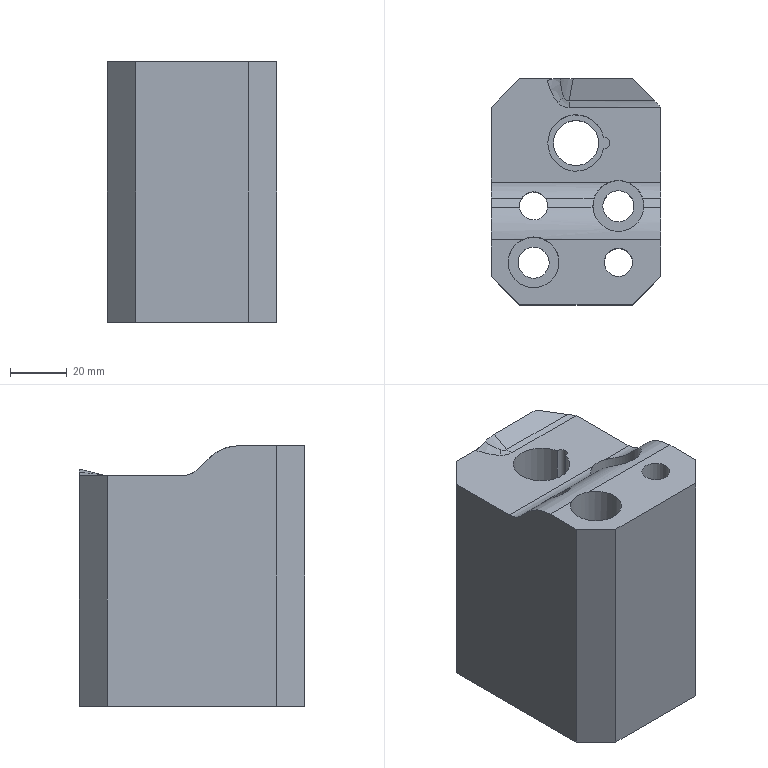Part | NX | features solid 2 | 1 solid | 37 faces | box 60 x 80 x 92.308 mm | volume 319167 mm3 | plane 19 | cylinder 15 | spline 3 | commonest cylinder face diameters 16 x3 20 x3 10 x2 11 x2 18 x2 4 x1
STEP:
#1=CARTESIAN_POINT('',(150.,-440.,5.));
#2=VERTEX_POINT('',#1);
#3=CARTESIAN_POINT('',(150.,-440.,97.308));
#4=VERTEX_POINT('',#3);
#5=CARTESIAN_POINT('',(150.,-440.,10.));
#6=DIRECTION('',(0.,0.,1.));
#7=VECTOR('',#6,1000.);
#8=LINE('',#5,#7);
#9=EDGE_CURVE('',#2,#4,#8,.T.);
#10=ORIENTED_EDGE('',*,*,#9,.T.);
#11=CARTESIAN_POINT('',(110.,-440.,97.308));
#12=VERTEX_POINT('',#11);
#13=CARTESIAN_POINT('',(130.,-440.,97.308));
#14=DIRECTION('',(-1.,0.,0.));
#15=VECTOR('',#14,1000.);
#16=LINE('',#13,#15);
#17=EDGE_CURVE('',#4,#12,#16,.T.);
#18=ORIENTED_EDGE('',*,*,#17,.T.);
#19=CARTESIAN_POINT('',(110.,-440.,5.));
#20=VERTEX_POINT('',#19);
#21=CARTESIAN_POINT('',(110.,-440.,10.));
#22=DIRECTION('',(0.,0.,-1.));
#23=VECTOR('',#22,1000.);
#24=LINE('',#21,#23);
#25=EDGE_CURVE('',#12,#20,#24,.T.);
#26=ORIENTED_EDGE('',*,*,#25,.T.);
#27=CARTESIAN_POINT('',(130.,-440.,5.));
#28=DIRECTION('',(-1.,0.,0.));
#29=VECTOR('',#28,1000.);
#30=LINE('',#27,#29);
#31=EDGE_CURVE('',#2,#20,#30,.T.);
#32=ORIENTED_EDGE('',*,*,#31,.F.);
#33=EDGE_LOOP('',(#10,#18,#26,#32));
#34=FACE_BOUND('',#33,.T.);
#35=CARTESIAN_POINT('',(130.,-440.,10.));
#36=DIRECTION('',(0.,-1.,0.));
#37=DIRECTION('',(0.,0.,-1.));
#38=AXIS2_PLACEMENT_3D('',#35,#36,#37);
#39=PLANE('',#38);
#40=ADVANCED_FACE('',(#34),#39,.T.);
#41=CARTESIAN_POINT('',(110.,-360.,5.));
#42=VERTEX_POINT('',#41);
#43=CARTESIAN_POINT('',(110.,-360.,86.708));
#44=VERTEX_POINT('',#43);
#45=CARTESIAN_POINT('',(110.,-360.,10.));
#46=DIRECTION('',(0.,0.,1.));
#47=VECTOR('',#46,1000.);
#48=LINE('',#45,#47);
#49=EDGE_CURVE('',#42,#44,#48,.T.);
#50=ORIENTED_EDGE('',*,*,#49,.T.);
#51=CARTESIAN_POINT('',(119.594,-360.,86.708));
#52=VERTEX_POINT('',#51);
#53=CARTESIAN_POINT('',(130.,-360.,86.708));
#54=DIRECTION('',(1.,0.,0.));
#55=VECTOR('',#54,1000.);
#56=LINE('',#53,#55);
#57=EDGE_CURVE('',#44,#52,#56,.T.);
#58=ORIENTED_EDGE('',*,*,#57,.T.);
#59=CARTESIAN_POINT('',(121.87,-360.,86.952));
#60=VERTEX_POINT('',#59);
#61=CARTESIAN_POINT('',(119.594,-360.,86.708));
#62=CARTESIAN_POINT('',(120.362,-360.,86.708));
#63=CARTESIAN_POINT('',(121.12,-360.,86.789));
#64=CARTESIAN_POINT('',(121.87,-360.,86.952));
#65=B_SPLINE_CURVE_WITH_KNOTS('',3,(#61,#62,#63,#64),.UNSPECIFIED.,.F.,.F.,(4,4),(0.,0.002289),.UNSPECIFIED.);
#66=EDGE_CURVE('',#52,#60,#65,.T.);
#67=ORIENTED_EDGE('',*,*,#66,.T.);
#68=CARTESIAN_POINT('',(124.411,-360.,87.846));
#69=VERTEX_POINT('',#68);
#70=CARTESIAN_POINT('',(121.87,-360.,86.952));
#71=CARTESIAN_POINT('',(122.751,-360.,87.142));
#72=CARTESIAN_POINT('',(123.605,-360.,87.443));
#73=CARTESIAN_POINT('',(124.411,-360.,87.846));
#74=B_SPLINE_CURVE_WITH_KNOTS('',3,(#70,#71,#72,#73),.UNSPECIFIED.,.F.,.F.,(4,4),(0.,0.002699),.UNSPECIFIED.);
#75=EDGE_CURVE('',#60,#69,#74,.T.);
#76=ORIENTED_EDGE('',*,*,#75,.T.);
#77=CARTESIAN_POINT('',(129.046,-360.,88.952));
#78=VERTEX_POINT('',#77);
#79=CARTESIAN_POINT('',(128.58,-360.,78.645));
#80=DIRECTION('',(0.,1.,0.));
#81=DIRECTION('',(0.6116,0.,0.7911));
#82=AXIS2_PLACEMENT_3D('',#79,#80,#81);
#83=ELLIPSE('',#82,10.485,10.);
#84=EDGE_CURVE('',#69,#78,#83,.T.);
#85=ORIENTED_EDGE('',*,*,#84,.T.);
#86=CARTESIAN_POINT('',(150.,-360.,88.952));
#87=VERTEX_POINT('',#86);
#88=CARTESIAN_POINT('',(130.,-360.,88.952));
#89=DIRECTION('',(-1.,0.,0.));
#90=VECTOR('',#89,1000.);
#91=LINE('',#88,#90);
#92=EDGE_CURVE('',#87,#78,#91,.T.);
#93=ORIENTED_EDGE('',*,*,#92,.F.);
#94=CARTESIAN_POINT('',(150.,-360.,5.));
#95=VERTEX_POINT('',#94);
#96=CARTESIAN_POINT('',(150.,-360.,10.));
#97=DIRECTION('',(0.,0.,-1.));
#98=VECTOR('',#97,1000.);
#99=LINE('',#96,#98);
#100=EDGE_CURVE('',#87,#95,#99,.T.);
#101=ORIENTED_EDGE('',*,*,#100,.T.);
#102=CARTESIAN_POINT('',(130.,-360.,5.));
#103=DIRECTION('',(1.,0.,0.));
#104=VECTOR('',#103,1000.);
#105=LINE('',#102,#104);
#106=EDGE_CURVE('',#42,#95,#105,.T.);
#107=ORIENTED_EDGE('',*,*,#106,.F.);
#108=EDGE_LOOP('',(#50,#58,#67,#76,#85,#93,#101,#107));
#109=FACE_BOUND('',#108,.T.);
#110=CARTESIAN_POINT('',(130.,-360.,10.));
#111=DIRECTION('',(0.,1.,0.));
#112=DIRECTION('',(0.,0.,1.));
#113=AXIS2_PLACEMENT_3D('',#110,#111,#112);
#114=PLANE('',#113);
#115=ADVANCED_FACE('',(#109),#114,.T.);
#116=CARTESIAN_POINT('',(100.,-430.,5.));
#117=VERTEX_POINT('',#116);
#118=CARTESIAN_POINT('',(100.,-430.,97.308));
#119=VERTEX_POINT('',#118);
#120=CARTESIAN_POINT('',(100.,-430.,10.));
#121=DIRECTION('',(0.,0.,1.));
#122=VECTOR('',#121,1000.);
#123=LINE('',#120,#122);
#124=EDGE_CURVE('',#117,#119,#123,.T.);
#125=ORIENTED_EDGE('',*,*,#124,.T.);
#126=CARTESIAN_POINT('',(100.,-417.041,97.308));
#127=VERTEX_POINT('',#126);
#128=CARTESIAN_POINT('',(100.,-360.,97.308));
#129=DIRECTION('',(0.,1.,0.));
#130=VECTOR('',#129,1000.);
#131=LINE('',#128,#130);
#132=EDGE_CURVE('',#119,#127,#131,.T.);
#133=ORIENTED_EDGE('',*,*,#132,.T.);
#134=CARTESIAN_POINT('',(100.,-405.652,92.546));
#135=VERTEX_POINT('',#134);
#136=CARTESIAN_POINT('',(100.,-417.041,81.308));
#137=DIRECTION('',(-1.,0.,0.));
#138=DIRECTION('',(0.,0.,1.));
#139=AXIS2_PLACEMENT_3D('',#136,#137,#138);
#140=CIRCLE('',#139,16.);
#141=EDGE_CURVE('',#127,#135,#140,.T.);
#142=ORIENTED_EDGE('',*,*,#141,.T.);
#143=CARTESIAN_POINT('',(100.,-402.24,89.089));
#144=VERTEX_POINT('',#143);
#145=CARTESIAN_POINT('',(100.,-341.861,27.899));
#146=DIRECTION('',(0.,-0.7024,0.7118));
#147=VECTOR('',#146,1000.);
#148=LINE('',#145,#147);
#149=EDGE_CURVE('',#144,#135,#148,.T.);
#150=ORIENTED_EDGE('',*,*,#149,.F.);
#151=CARTESIAN_POINT('',(100.,-396.546,86.708));
#152=VERTEX_POINT('',#151);
#153=CARTESIAN_POINT('',(100.,-396.546,94.708));
#154=DIRECTION('',(-1.,0.,0.));
#155=DIRECTION('',(0.,0.,1.));
#156=AXIS2_PLACEMENT_3D('',#153,#154,#155);
#157=CIRCLE('',#156,8.);
#158=EDGE_CURVE('',#152,#144,#157,.T.);
#159=ORIENTED_EDGE('',*,*,#158,.F.);
#160=CARTESIAN_POINT('',(100.,-370.,86.708));
#161=VERTEX_POINT('',#160);
#162=CARTESIAN_POINT('',(100.,-360.,86.708));
#163=DIRECTION('',(0.,1.,0.));
#164=VECTOR('',#163,1000.);
#165=LINE('',#162,#164);
#166=EDGE_CURVE('',#152,#161,#165,.T.);
#167=ORIENTED_EDGE('',*,*,#166,.T.);
#168=CARTESIAN_POINT('',(100.,-370.,5.));
#169=VERTEX_POINT('',#168);
#170=CARTESIAN_POINT('',(100.,-370.,10.));
#171=DIRECTION('',(0.,0.,-1.));
#172=VECTOR('',#171,1000.);
#173=LINE('',#170,#172);
#174=EDGE_CURVE('',#161,#169,#173,.T.);
#175=ORIENTED_EDGE('',*,*,#174,.T.);
#176=CARTESIAN_POINT('',(100.,-360.,5.));
#177=DIRECTION('',(0.,1.,0.));
#178=VECTOR('',#177,1000.);
#179=LINE('',#176,#178);
#180=EDGE_CURVE('',#117,#169,#179,.T.);
#181=ORIENTED_EDGE('',*,*,#180,.F.);
#182=EDGE_LOOP('',(#125,#133,#142,#150,#159,#167,#175,#181));
#183=FACE_BOUND('',#182,.T.);
#184=CARTESIAN_POINT('',(100.,-360.,10.));
#185=DIRECTION('',(-1.,0.,0.));
#186=DIRECTION('',(0.,0.,-1.));
#187=AXIS2_PLACEMENT_3D('',#184,#185,#186);
#188=PLANE('',#187);
#189=ADVANCED_FACE('',(#183),#188,.T.);
#190=ORIENTED_EDGE('',*,*,#174,.F.);
#191=CARTESIAN_POINT('',(110.,-360.,86.708));
#192=DIRECTION('',(-0.7071,-0.7071,0.));
#193=VECTOR('',#192,1000.);
#194=LINE('',#191,#193);
#195=EDGE_CURVE('',#161,#44,#194,.F.);
#196=ORIENTED_EDGE('',*,*,#195,.T.);
#197=ORIENTED_EDGE('',*,*,#49,.F.);
#198=CARTESIAN_POINT('',(120.,-350.,5.));
#199=DIRECTION('',(-0.7071,-0.7071,0.));
#200=VECTOR('',#199,1000.);
#201=LINE('',#198,#200);
#202=EDGE_CURVE('',#169,#42,#201,.F.);
#203=ORIENTED_EDGE('',*,*,#202,.F.);
#204=EDGE_LOOP('',(#190,#196,#197,#203));
#205=FACE_BOUND('',#204,.T.);
#206=CARTESIAN_POINT('',(110.,-360.,10.));
#207=DIRECTION('',(0.7071,-0.7071,0.));
#208=DIRECTION('',(0.7071,0.7071,0.));
#209=AXIS2_PLACEMENT_3D('',#206,#207,#208);
#210=PLANE('',#209);
#211=ADVANCED_FACE('',(#205),#210,.F.);
#212=CARTESIAN_POINT('',(160.,-430.,97.308));
#213=VERTEX_POINT('',#212);
#214=CARTESIAN_POINT('',(160.,-430.,5.));
#215=VERTEX_POINT('',#214);
#216=CARTESIAN_POINT('',(160.,-430.,10.));
#217=DIRECTION('',(0.,0.,-1.));
#218=VECTOR('',#217,1000.);
#219=LINE('',#216,#218);
#220=EDGE_CURVE('',#213,#215,#219,.T.);
#221=ORIENTED_EDGE('',*,*,#220,.F.);
#222=CARTESIAN_POINT('',(150.,-440.,97.308));
#223=DIRECTION('',(0.7071,0.7071,0.));
#224=VECTOR('',#223,1000.);
#225=LINE('',#222,#224);
#226=EDGE_CURVE('',#213,#4,#225,.F.);
#227=ORIENTED_EDGE('',*,*,#226,.T.);
#228=ORIENTED_EDGE('',*,*,#9,.F.);
#229=CARTESIAN_POINT('',(180.,-410.,5.));
#230=DIRECTION('',(0.7071,0.7071,0.));
#231=VECTOR('',#230,1000.);
#232=LINE('',#229,#231);
#233=EDGE_CURVE('',#215,#2,#232,.F.);
#234=ORIENTED_EDGE('',*,*,#233,.F.);
#235=EDGE_LOOP('',(#221,#227,#228,#234));
#236=FACE_BOUND('',#235,.T.);
#237=CARTESIAN_POINT('',(150.,-440.,10.));
#238=DIRECTION('',(-0.7071,0.7071,0.));
#239=DIRECTION('',(-0.7071,-0.7071,0.));
#240=AXIS2_PLACEMENT_3D('',#237,#238,#239);
#241=PLANE('',#240);
#242=ADVANCED_FACE('',(#236),#241,.F.);
#243=ORIENTED_EDGE('',*,*,#25,.F.);
#244=CARTESIAN_POINT('',(100.,-430.,97.308));
#245=DIRECTION('',(0.7071,-0.7071,0.));
#246=VECTOR('',#245,1000.);
#247=LINE('',#244,#246);
#248=EDGE_CURVE('',#12,#119,#247,.F.);
#249=ORIENTED_EDGE('',*,*,#248,.T.);
#250=ORIENTED_EDGE('',*,*,#124,.F.);
#251=CARTESIAN_POINT('',(80.,-410.,5.));
#252=DIRECTION('',(0.7071,-0.7071,0.));
#253=VECTOR('',#252,1000.);
#254=LINE('',#251,#253);
#255=EDGE_CURVE('',#20,#117,#254,.F.);
#256=ORIENTED_EDGE('',*,*,#255,.F.);
#257=EDGE_LOOP('',(#243,#249,#250,#256));
#258=FACE_BOUND('',#257,.T.);
#259=CARTESIAN_POINT('',(100.,-430.,10.));
#260=DIRECTION('',(0.7071,0.7071,0.));
#261=DIRECTION('',(-0.7071,0.7071,0.));
#262=AXIS2_PLACEMENT_3D('',#259,#260,#261);
#263=PLANE('',#262);
#264=ADVANCED_FACE('',(#258),#263,.F.);
#265=CARTESIAN_POINT('',(106.,-425.,35.));
#266=VERTEX_POINT('',#265);
#267=CARTESIAN_POINT('',(115.,-425.,35.));
#268=DIRECTION('',(0.,0.,-1.));
#269=DIRECTION('',(-1.,0.,0.));
#270=AXIS2_PLACEMENT_3D('',#267,#268,#269);
#271=CIRCLE('',#270,9.);
#272=EDGE_CURVE('',#266,#266,#271,.T.);
#273=ORIENTED_EDGE('',*,*,#272,.T.);
#274=EDGE_LOOP('',(#273));
#275=FACE_BOUND('',#274,.T.);
#276=CARTESIAN_POINT('',(119.201,-417.041,97.308));
#277=VERTEX_POINT('',#276);
#278=CARTESIAN_POINT('',(110.799,-417.041,97.308));
#279=VERTEX_POINT('',#278);
#280=CARTESIAN_POINT('',(115.,-425.,97.308));
#281=DIRECTION('',(0.,0.,1.));
#282=DIRECTION('',(1.,0.,0.));
#283=AXIS2_PLACEMENT_3D('',#280,#281,#282);
#284=CIRCLE('',#283,9.);
#285=EDGE_CURVE('',#277,#279,#284,.F.);
#286=ORIENTED_EDGE('',*,*,#285,.F.);
#287=CARTESIAN_POINT('',(110.799,-417.041,97.308));
#288=CARTESIAN_POINT('',(112.099,-416.354,97.308));
#289=CARTESIAN_POINT('',(114.996,-415.646,97.24));
#290=CARTESIAN_POINT('',(117.901,-416.354,97.308));
#291=CARTESIAN_POINT('',(119.201,-417.041,97.308));
#292=B_SPLINE_CURVE_WITH_KNOTS('',3,(#287,#288,#289,#290,#291),.UNSPECIFIED.,.F.,.F.,(4,1,4),(0.,0.004347,0.008695),.UNSPECIFIED.);
#293=EDGE_CURVE('',#279,#277,#292,.T.);
#294=ORIENTED_EDGE('',*,*,#293,.F.);
#295=EDGE_LOOP('',(#286,#294));
#296=FACE_BOUND('',#295,.T.);
#297=CARTESIAN_POINT('',(115.,-425.,110.));
#298=DIRECTION('',(0.,0.,-1.));
#299=DIRECTION('',(-1.,0.,0.));
#300=AXIS2_PLACEMENT_3D('',#297,#298,#299);
#301=CYLINDRICAL_SURFACE('',#300,9.);
#302=ADVANCED_FACE('',(#275,#296),#301,.F.);
#303=CARTESIAN_POINT('',(140.,-425.,5.));
#304=VERTEX_POINT('',#303);
#305=CARTESIAN_POINT('',(145.,-425.,5.));
#306=DIRECTION('',(0.,0.,-1.));
#307=DIRECTION('',(-1.,0.,0.));
#308=AXIS2_PLACEMENT_3D('',#305,#306,#307);
#309=CIRCLE('',#308,5.);
#310=EDGE_CURVE('',#304,#304,#309,.T.);
#311=ORIENTED_EDGE('',*,*,#310,.T.);
#312=EDGE_LOOP('',(#311));
#313=FACE_BOUND('',#312,.T.);
#314=CARTESIAN_POINT('',(150.,-425.,97.308));
#315=VERTEX_POINT('',#314);
#316=CARTESIAN_POINT('',(145.,-425.,97.308));
#317=DIRECTION('',(0.,0.,1.));
#318=DIRECTION('',(1.,0.,0.));
#319=AXIS2_PLACEMENT_3D('',#316,#317,#318);
#320=CIRCLE('',#319,5.);
#321=EDGE_CURVE('',#315,#315,#320,.F.);
#322=ORIENTED_EDGE('',*,*,#321,.F.);
#323=EDGE_LOOP('',(#322));
#324=FACE_BOUND('',#323,.T.);
#325=CARTESIAN_POINT('',(145.,-425.,110.));
#326=DIRECTION('',(0.,0.,-1.));
#327=DIRECTION('',(-1.,0.,0.));
#328=AXIS2_PLACEMENT_3D('',#325,#326,#327);
#329=CYLINDRICAL_SURFACE('',#328,5.);
#330=ADVANCED_FACE('',(#313,#324),#329,.F.);
#331=CARTESIAN_POINT('',(160.,-370.228,86.708));
#332=VERTEX_POINT('',#331);
#333=CARTESIAN_POINT('',(160.,-370.,86.71));
#334=VERTEX_POINT('',#333);
#335=CARTESIAN_POINT('',(160.,-370.228,96.708));
#336=DIRECTION('',(1.,0.,0.));
#337=DIRECTION('',(0.,0.,-1.));
#338=AXIS2_PLACEMENT_3D('',#335,#336,#337);
#339=CIRCLE('',#338,10.);
#340=EDGE_CURVE('',#332,#334,#339,.T.);
#341=ORIENTED_EDGE('',*,*,#340,.F.);
#342=CARTESIAN_POINT('',(160.,-396.546,86.708));
#343=VERTEX_POINT('',#342);
#344=CARTESIAN_POINT('',(160.,-360.,86.708));
#345=DIRECTION('',(0.,-1.,0.));
#346=VECTOR('',#345,1000.);
#347=LINE('',#344,#346);
#348=EDGE_CURVE('',#332,#343,#347,.T.);
#349=ORIENTED_EDGE('',*,*,#348,.T.);
#350=CARTESIAN_POINT('',(160.,-402.24,89.089));
#351=VERTEX_POINT('',#350);
#352=CARTESIAN_POINT('',(160.,-396.546,94.708));
#353=DIRECTION('',(1.,0.,0.));
#354=DIRECTION('',(0.,0.,-1.));
#355=AXIS2_PLACEMENT_3D('',#352,#353,#354);
#356=CIRCLE('',#355,8.);
#357=EDGE_CURVE('',#351,#343,#356,.T.);
#358=ORIENTED_EDGE('',*,*,#357,.F.);
#359=CARTESIAN_POINT('',(160.,-405.652,92.546));
#360=VERTEX_POINT('',#359);
#361=CARTESIAN_POINT('',(160.,-341.861,27.899));
#362=DIRECTION('',(0.,0.7024,-0.7118));
#363=VECTOR('',#362,1000.);
#364=LINE('',#361,#363);
#365=EDGE_CURVE('',#360,#351,#364,.T.);
#366=ORIENTED_EDGE('',*,*,#365,.F.);
#367=CARTESIAN_POINT('',(160.,-417.041,97.308));
#368=VERTEX_POINT('',#367);
#369=CARTESIAN_POINT('',(160.,-417.041,81.308));
#370=DIRECTION('',(1.,0.,0.));
#371=DIRECTION('',(0.,0.,-1.));
#372=AXIS2_PLACEMENT_3D('',#369,#370,#371);
#373=CIRCLE('',#372,16.);
#374=EDGE_CURVE('',#360,#368,#373,.T.);
#375=ORIENTED_EDGE('',*,*,#374,.T.);
#376=CARTESIAN_POINT('',(160.,-360.,97.308));
#377=DIRECTION('',(0.,-1.,0.));
#378=VECTOR('',#377,1000.);
#379=LINE('',#376,#378);
#380=EDGE_CURVE('',#368,#213,#379,.T.);
#381=ORIENTED_EDGE('',*,*,#380,.T.);
#382=ORIENTED_EDGE('',*,*,#220,.T.);
#383=CARTESIAN_POINT('',(160.,-370.,5.));
#384=VERTEX_POINT('',#383);
#385=CARTESIAN_POINT('',(160.,-360.,5.));
#386=DIRECTION('',(0.,-1.,0.));
#387=VECTOR('',#386,1000.);
#388=LINE('',#385,#387);
#389=EDGE_CURVE('',#384,#215,#388,.T.);
#390=ORIENTED_EDGE('',*,*,#389,.F.);
#391=CARTESIAN_POINT('',(160.,-370.,10.));
#392=DIRECTION('',(0.,0.,1.));
#393=VECTOR('',#392,1000.);
#394=LINE('',#391,#393);
#395=EDGE_CURVE('',#384,#334,#394,.T.);
#396=ORIENTED_EDGE('',*,*,#395,.T.);
#397=EDGE_LOOP('',(#341,#349,#358,#366,#375,#381,#382,#390,#396));
#398=FACE_BOUND('',#397,.T.);
#399=CARTESIAN_POINT('',(160.,-360.,10.));
#400=DIRECTION('',(1.,0.,0.));
#401=DIRECTION('',(0.,0.,1.));
#402=AXIS2_PLACEMENT_3D('',#399,#400,#401);
#403=PLANE('',#402);
#404=ADVANCED_FACE('',(#398),#403,.T.);
#405=CARTESIAN_POINT('',(118.511,-382.715,5.));
#406=VERTEX_POINT('',#405);
#407=CARTESIAN_POINT('',(130.011,-382.715,5.));
#408=DIRECTION('',(0.,0.,-1.));
#409=DIRECTION('',(-1.,0.,0.));
#410=AXIS2_PLACEMENT_3D('',#407,#408,#409);
#411=CIRCLE('',#410,11.5);
#412=EDGE_CURVE('',#406,#406,#411,.F.);
#413=ORIENTED_EDGE('',*,*,#412,.T.);
#414=EDGE_LOOP('',(#413));
#415=FACE_BOUND('',#414,.T.);
#416=ORIENTED_EDGE('',*,*,#310,.F.);
#417=EDGE_LOOP('',(#416));
#418=FACE_BOUND('',#417,.T.);
#419=CARTESIAN_POINT('',(110.,-405.,5.));
#420=VERTEX_POINT('',#419);
#421=CARTESIAN_POINT('',(115.,-405.,5.));
#422=DIRECTION('',(0.,0.,-1.));
#423=DIRECTION('',(-1.,0.,0.));
#424=AXIS2_PLACEMENT_3D('',#421,#422,#423);
#425=CIRCLE('',#424,5.);
#426=EDGE_CURVE('',#420,#420,#425,.T.);
#427=ORIENTED_EDGE('',*,*,#426,.F.);
#428=EDGE_LOOP('',(#427));
#429=FACE_BOUND('',#428,.T.);
#430=CARTESIAN_POINT('',(139.5,-405.,5.));
#431=VERTEX_POINT('',#430);
#432=CARTESIAN_POINT('',(145.,-405.,5.));
#433=DIRECTION('',(0.,0.,-1.));
#434=DIRECTION('',(-1.,0.,0.));
#435=AXIS2_PLACEMENT_3D('',#432,#433,#434);
#436=CIRCLE('',#435,5.5);
#437=EDGE_CURVE('',#431,#431,#436,.T.);
#438=ORIENTED_EDGE('',*,*,#437,.F.);
#439=EDGE_LOOP('',(#438));
#440=FACE_BOUND('',#439,.T.);
#441=CARTESIAN_POINT('',(109.5,-425.,5.));
#442=VERTEX_POINT('',#441);
#443=CARTESIAN_POINT('',(115.,-425.,5.));
#444=DIRECTION('',(0.,0.,-1.));
#445=DIRECTION('',(-1.,0.,0.));
#446=AXIS2_PLACEMENT_3D('',#443,#444,#445);
#447=CIRCLE('',#446,5.5);
#448=EDGE_CURVE('',#442,#442,#447,.T.);
#449=ORIENTED_EDGE('',*,*,#448,.F.);
#450=EDGE_LOOP('',(#449));
#451=FACE_BOUND('',#450,.T.);
#452=ORIENTED_EDGE('',*,*,#180,.T.);
#453=ORIENTED_EDGE('',*,*,#202,.T.);
#454=ORIENTED_EDGE('',*,*,#106,.T.);
#455=CARTESIAN_POINT('',(140.,-350.,5.));
#456=DIRECTION('',(-0.7071,0.7071,0.));
#457=VECTOR('',#456,1000.);
#458=LINE('',#455,#457);
#459=EDGE_CURVE('',#95,#384,#458,.F.);
#460=ORIENTED_EDGE('',*,*,#459,.T.);
#461=ORIENTED_EDGE('',*,*,#389,.T.);
#462=ORIENTED_EDGE('',*,*,#233,.T.);
#463=ORIENTED_EDGE('',*,*,#31,.T.);
#464=ORIENTED_EDGE('',*,*,#255,.T.);
#465=EDGE_LOOP('',(#452,#453,#454,#460,#461,#462,#463,#464));
#466=FACE_BOUND('',#465,.T.);
#467=CARTESIAN_POINT('',(130.,-360.,5.));
#468=DIRECTION('',(0.,0.,-1.));
#469=DIRECTION('',(1.,0.,0.));
#470=AXIS2_PLACEMENT_3D('',#467,#468,#469);
#471=PLANE('',#470);
#472=ADVANCED_FACE('',(#415,#418,#429,#440,#451,#466),#471,.T.);
#473=CARTESIAN_POINT('',(157.809,-367.809,87.005));
#474=VERTEX_POINT('',#473);
#475=CARTESIAN_POINT('',(160.228,-370.228,96.708));
#476=DIRECTION('',(-0.7071,-0.7071,0.));
#477=DIRECTION('',(-0.7071,0.7071,0.));
#478=AXIS2_PLACEMENT_3D('',#475,#476,#477);
#479=ELLIPSE('',#478,14.142,10.);
#480=EDGE_CURVE('',#334,#474,#479,.F.);
#481=ORIENTED_EDGE('',*,*,#480,.F.);
#482=ORIENTED_EDGE('',*,*,#395,.F.);
#483=ORIENTED_EDGE('',*,*,#459,.F.);
#484=ORIENTED_EDGE('',*,*,#100,.F.);
#485=CARTESIAN_POINT('',(169.244,-379.244,84.153));
#486=DIRECTION('',(0.6964,-0.6964,-0.1736));
#487=VECTOR('',#486,1000.);
#488=LINE('',#485,#487);
#489=EDGE_CURVE('',#474,#87,#488,.F.);
#490=ORIENTED_EDGE('',*,*,#489,.F.);
#491=EDGE_LOOP('',(#481,#482,#483,#484,#490));
#492=FACE_BOUND('',#491,.T.);
#493=CARTESIAN_POINT('',(160.,-370.,10.));
#494=DIRECTION('',(-0.7071,-0.7071,0.));
#495=DIRECTION('',(0.7071,-0.7071,0.));
#496=AXIS2_PLACEMENT_3D('',#493,#494,#495);
#497=PLANE('',#496);
#498=ADVANCED_FACE('',(#492),#497,.F.);
#499=ORIENTED_EDGE('',*,*,#448,.T.);
#500=EDGE_LOOP('',(#499));
#501=FACE_BOUND('',#500,.T.);
#502=CARTESIAN_POINT('',(109.5,-425.,35.));
#503=VERTEX_POINT('',#502);
#504=CARTESIAN_POINT('',(115.,-425.,35.));
#505=DIRECTION('',(0.,0.,-1.));
#506=DIRECTION('',(-1.,0.,0.));
#507=AXIS2_PLACEMENT_3D('',#504,#505,#506);
#508=CIRCLE('',#507,5.5);
#509=EDGE_CURVE('',#503,#503,#508,.T.);
#510=ORIENTED_EDGE('',*,*,#509,.F.);
#511=EDGE_LOOP('',(#510));
#512=FACE_BOUND('',#511,.T.);
#513=CARTESIAN_POINT('',(115.,-425.,5.));
#514=DIRECTION('',(0.,0.,-1.));
#515=DIRECTION('',(-1.,0.,0.));
#516=AXIS2_PLACEMENT_3D('',#513,#514,#515);
#517=CYLINDRICAL_SURFACE('',#516,5.5);
#518=ADVANCED_FACE('',(#501,#512),#517,.F.);
#519=ORIENTED_EDGE('',*,*,#509,.T.);
#520=EDGE_LOOP('',(#519));
#521=FACE_BOUND('',#520,.T.);
#522=ORIENTED_EDGE('',*,*,#272,.F.);
#523=EDGE_LOOP('',(#522));
#524=FACE_BOUND('',#523,.T.);
#525=CARTESIAN_POINT('',(115.,-425.,35.));
#526=DIRECTION('',(0.,0.,-1.));
#527=DIRECTION('',(-1.,0.,0.));
#528=AXIS2_PLACEMENT_3D('',#525,#526,#527);
#529=PLANE('',#528);
#530=ADVANCED_FACE('',(#521,#524),#529,.F.);
#531=ORIENTED_EDGE('',*,*,#437,.T.);
#532=EDGE_LOOP('',(#531));
#533=FACE_BOUND('',#532,.T.);
#534=CARTESIAN_POINT('',(139.5,-405.,35.));
#535=VERTEX_POINT('',#534);
#536=CARTESIAN_POINT('',(145.,-405.,35.));
#537=DIRECTION('',(0.,0.,-1.));
#538=DIRECTION('',(-1.,0.,0.));
#539=AXIS2_PLACEMENT_3D('',#536,#537,#538);
#540=CIRCLE('',#539,5.5);
#541=EDGE_CURVE('',#535,#535,#540,.T.);
#542=ORIENTED_EDGE('',*,*,#541,.F.);
#543=EDGE_LOOP('',(#542));
#544=FACE_BOUND('',#543,.T.);
#545=CARTESIAN_POINT('',(145.,-405.,5.));
#546=DIRECTION('',(0.,0.,-1.));
#547=DIRECTION('',(-1.,0.,0.));
#548=AXIS2_PLACEMENT_3D('',#545,#546,#547);
#549=CYLINDRICAL_SURFACE('',#548,5.5);
#550=ADVANCED_FACE('',(#533,#544),#549,.F.);
#551=ORIENTED_EDGE('',*,*,#541,.T.);
#552=EDGE_LOOP('',(#551));
#553=FACE_BOUND('',#552,.T.);
#554=CARTESIAN_POINT('',(136.,-405.,35.));
#555=VERTEX_POINT('',#554);
#556=CARTESIAN_POINT('',(145.,-405.,35.));
#557=DIRECTION('',(0.,0.,-1.));
#558=DIRECTION('',(-1.,0.,0.));
#559=AXIS2_PLACEMENT_3D('',#556,#557,#558);
#560=CIRCLE('',#559,9.);
#561=EDGE_CURVE('',#555,#555,#560,.T.);
#562=ORIENTED_EDGE('',*,*,#561,.F.);
#563=EDGE_LOOP('',(#562));
#564=FACE_BOUND('',#563,.T.);
#565=CARTESIAN_POINT('',(145.,-405.,35.));
#566=DIRECTION('',(0.,0.,-1.));
#567=DIRECTION('',(-1.,0.,0.));
#568=AXIS2_PLACEMENT_3D('',#565,#566,#567);
#569=PLANE('',#568);
#570=ADVANCED_FACE('',(#553,#564),#569,.F.);
#571=CARTESIAN_POINT('',(141.913,-396.546,86.708));
#572=VERTEX_POINT('',#571);
#573=CARTESIAN_POINT('',(148.087,-396.546,86.708));
#574=VERTEX_POINT('',#573);
#575=CARTESIAN_POINT('',(145.,-405.,86.708));
#576=DIRECTION('',(0.,0.,1.));
#577=DIRECTION('',(1.,0.,0.));
#578=AXIS2_PLACEMENT_3D('',#575,#576,#577);
#579=CIRCLE('',#578,9.);
#580=EDGE_CURVE('',#572,#574,#579,.F.);
#581=ORIENTED_EDGE('',*,*,#580,.F.);
#582=CARTESIAN_POINT('',(136.434,-402.24,89.089));
#583=VERTEX_POINT('',#582);
#584=CARTESIAN_POINT('',(141.913,-396.546,86.708));
#585=CARTESIAN_POINT('',(140.531,-397.051,86.708));
#586=CARTESIAN_POINT('',(138.034,-398.754,86.767));
#587=CARTESIAN_POINT('',(136.759,-401.229,88.064));
#588=CARTESIAN_POINT('',(136.434,-402.24,89.089));
#589=B_SPLINE_CURVE_WITH_KNOTS('',3,(#584,#585,#586,#587,#588),.UNSPECIFIED.,.F.,.F.,(4,1,4),(0.,0.004358,0.008716),.UNSPECIFIED.);
#590=EDGE_CURVE('',#572,#583,#589,.T.);
#591=ORIENTED_EDGE('',*,*,#590,.T.);
#592=CARTESIAN_POINT('',(136.024,-405.652,92.546));
#593=VERTEX_POINT('',#592);
#594=CARTESIAN_POINT('',(145.,-405.,91.885));
#595=DIRECTION('',(0.,-0.7118,-0.7024));
#596=DIRECTION('',(0.,0.7024,-0.7118));
#597=AXIS2_PLACEMENT_3D('',#594,#595,#596);
#598=ELLIPSE('',#597,12.814,9.);
#599=EDGE_CURVE('',#583,#593,#598,.F.);
#600=ORIENTED_EDGE('',*,*,#599,.T.);
#601=CARTESIAN_POINT('',(153.976,-405.652,92.546));
#602=VERTEX_POINT('',#601);
#603=CARTESIAN_POINT('',(153.976,-405.652,92.546));
#604=CARTESIAN_POINT('',(153.914,-406.513,93.419));
#605=CARTESIAN_POINT('',(153.527,-408.421,94.941));
#606=CARTESIAN_POINT('',(151.701,-411.359,96.352));
#607=CARTESIAN_POINT('',(148.672,-413.492,96.93));
#608=CARTESIAN_POINT('',(145.017,-414.251,97.058));
#609=CARTESIAN_POINT('',(141.353,-413.503,96.933));
#610=CARTESIAN_POINT('',(138.315,-411.377,96.358));
#611=CARTESIAN_POINT('',(136.476,-408.434,94.95));
#612=CARTESIAN_POINT('',(136.086,-406.514,93.42));
#613=CARTESIAN_POINT('',(136.024,-405.652,92.546));
#614=B_SPLINE_CURVE_WITH_KNOTS('',3,(#603,#604,#605,#606,#607,#608,#609,#610,#611,#612,#613),.UNSPECIFIED.,.F.,.F.,(4,1,1,1,1,1,1,1,4),(0.,0.003639,0.007278,0.01092,0.01456,0.01819,0.02183,0.02547,0.02911),.UNSPECIFIED.);
#615=EDGE_CURVE('',#602,#593,#614,.T.);
#616=ORIENTED_EDGE('',*,*,#615,.F.);
#617=CARTESIAN_POINT('',(153.566,-402.24,89.089));
#618=VERTEX_POINT('',#617);
#619=CARTESIAN_POINT('',(145.,-405.,91.885));
#620=DIRECTION('',(0.,-0.7118,-0.7024));
#621=DIRECTION('',(0.,0.7024,-0.7118));
#622=AXIS2_PLACEMENT_3D('',#619,#620,#621);
#623=ELLIPSE('',#622,12.814,9.);
#624=EDGE_CURVE('',#602,#618,#623,.F.);
#625=ORIENTED_EDGE('',*,*,#624,.T.);
#626=CARTESIAN_POINT('',(153.566,-402.24,89.089));
#627=CARTESIAN_POINT('',(153.242,-401.232,88.067));
#628=CARTESIAN_POINT('',(151.982,-398.77,86.771));
#629=CARTESIAN_POINT('',(149.467,-397.05,86.708));
#630=CARTESIAN_POINT('',(148.087,-396.546,86.708));
#631=B_SPLINE_CURVE_WITH_KNOTS('',3,(#626,#627,#628,#629,#630),.UNSPECIFIED.,.F.,.F.,(4,1,4),(0.,0.004352,0.008704),.UNSPECIFIED.);
#632=EDGE_CURVE('',#618,#574,#631,.T.);
#633=ORIENTED_EDGE('',*,*,#632,.T.);
#634=EDGE_LOOP('',(#581,#591,#600,#616,#625,#633));
#635=FACE_BOUND('',#634,.T.);
#636=ORIENTED_EDGE('',*,*,#561,.T.);
#637=EDGE_LOOP('',(#636));
#638=FACE_BOUND('',#637,.T.);
#639=CARTESIAN_POINT('',(145.,-405.,110.));
#640=DIRECTION('',(0.,0.,-1.));
#641=DIRECTION('',(-1.,0.,0.));
#642=AXIS2_PLACEMENT_3D('',#639,#640,#641);
#643=CYLINDRICAL_SURFACE('',#642,9.);
#644=ADVANCED_FACE('',(#635,#638),#643,.F.);
#645=CARTESIAN_POINT('',(119.169,-402.24,89.089));
#646=VERTEX_POINT('',#645);
#647=CARTESIAN_POINT('',(110.831,-402.24,89.089));
#648=VERTEX_POINT('',#647);
#649=CARTESIAN_POINT('',(119.169,-402.24,89.089));
#650=CARTESIAN_POINT('',(118.794,-401.674,88.514));
#651=CARTESIAN_POINT('',(117.655,-400.5,87.7));
#652=CARTESIAN_POINT('',(115.,-399.751,87.388));
#653=CARTESIAN_POINT('',(112.348,-400.498,87.699));
#654=CARTESIAN_POINT('',(111.206,-401.674,88.514));
#655=CARTESIAN_POINT('',(110.831,-402.24,89.089));
#656=B_SPLINE_CURVE_WITH_KNOTS('',3,(#649,#650,#651,#652,#653,#654,#655),.UNSPECIFIED.,.F.,.F.,(4,1,1,1,4),(0.,0.002634,0.005268,0.007902,0.01054),.UNSPECIFIED.);
#657=EDGE_CURVE('',#646,#648,#656,.T.);
#658=ORIENTED_EDGE('',*,*,#657,.T.);
#659=CARTESIAN_POINT('',(110.043,-405.652,92.546));
#660=VERTEX_POINT('',#659);
#661=CARTESIAN_POINT('',(115.,-405.,91.885));
#662=DIRECTION('',(0.,-0.7118,-0.7024));
#663=DIRECTION('',(0.,0.7024,-0.7118));
#664=AXIS2_PLACEMENT_3D('',#661,#662,#663);
#665=ELLIPSE('',#664,7.119,5.);
#666=EDGE_CURVE('',#648,#660,#665,.F.);
#667=ORIENTED_EDGE('',*,*,#666,.T.);
#668=CARTESIAN_POINT('',(119.957,-405.652,92.546));
#669=VERTEX_POINT('',#668);
#670=CARTESIAN_POINT('',(119.957,-405.652,92.546));
#671=CARTESIAN_POINT('',(119.833,-406.597,93.504));
#672=CARTESIAN_POINT('',(118.997,-408.762,95.124));
#673=CARTESIAN_POINT('',(115.011,-410.615,95.949));
#674=CARTESIAN_POINT('',(111.015,-408.779,95.134));
#675=CARTESIAN_POINT('',(110.167,-406.599,93.506));
#676=CARTESIAN_POINT('',(110.043,-405.652,92.546));
#677=B_SPLINE_CURVE_WITH_KNOTS('',3,(#670,#671,#672,#673,#674,#675,#676),.UNSPECIFIED.,.F.,.F.,(4,1,1,1,4),(0.,0.003993,0.007986,0.01198,0.01597),.UNSPECIFIED.);
#678=EDGE_CURVE('',#669,#660,#677,.T.);
#679=ORIENTED_EDGE('',*,*,#678,.F.);
#680=CARTESIAN_POINT('',(115.,-405.,91.885));
#681=DIRECTION('',(0.,-0.7118,-0.7024));
#682=DIRECTION('',(0.,0.7024,-0.7118));
#683=AXIS2_PLACEMENT_3D('',#680,#681,#682);
#684=ELLIPSE('',#683,7.119,5.);
#685=EDGE_CURVE('',#669,#646,#684,.F.);
#686=ORIENTED_EDGE('',*,*,#685,.T.);
#687=EDGE_LOOP('',(#658,#667,#679,#686));
#688=FACE_BOUND('',#687,.T.);
#689=ORIENTED_EDGE('',*,*,#426,.T.);
#690=EDGE_LOOP('',(#689));
#691=FACE_BOUND('',#690,.T.);
#692=CARTESIAN_POINT('',(115.,-405.,110.));
#693=DIRECTION('',(0.,0.,-1.));
#694=DIRECTION('',(-1.,0.,0.));
#695=AXIS2_PLACEMENT_3D('',#692,#693,#694);
#696=CYLINDRICAL_SURFACE('',#695,5.);
#697=ADVANCED_FACE('',(#688,#691),#696,.F.);
#698=CARTESIAN_POINT('',(139.811,-384.705,86.708));
#699=VERTEX_POINT('',#698);
#700=CARTESIAN_POINT('',(139.811,-380.725,86.708));
#701=VERTEX_POINT('',#700);
#702=CARTESIAN_POINT('',(140.011,-382.715,86.708));
#703=DIRECTION('',(0.,0.,1.));
#704=DIRECTION('',(1.,0.,0.));
#705=AXIS2_PLACEMENT_3D('',#702,#703,#704);
#706=CIRCLE('',#705,2.);
#707=EDGE_CURVE('',#699,#701,#706,.T.);
#708=ORIENTED_EDGE('',*,*,#707,.F.);
#709=CARTESIAN_POINT('',(130.011,-382.715,86.708));
#710=DIRECTION('',(0.,0.,1.));
#711=DIRECTION('',(1.,0.,0.));
#712=AXIS2_PLACEMENT_3D('',#709,#710,#711);
#713=CIRCLE('',#712,10.);
#714=EDGE_CURVE('',#699,#701,#713,.F.);
#715=ORIENTED_EDGE('',*,*,#714,.T.);
#716=EDGE_LOOP('',(#708,#715));
#717=FACE_BOUND('',#716,.T.);
#718=ORIENTED_EDGE('',*,*,#348,.F.);
#719=CARTESIAN_POINT('',(127.541,-370.228,86.708));
#720=VERTEX_POINT('',#719);
#721=CARTESIAN_POINT('',(160.,-370.228,86.708));
#722=CARTESIAN_POINT('',(149.18,-370.228,86.708));
#723=CARTESIAN_POINT('',(138.361,-370.228,86.708));
#724=CARTESIAN_POINT('',(127.541,-370.228,86.708));
#725=B_SPLINE_CURVE_WITH_KNOTS('',3,(#721,#722,#723,#724),.UNSPECIFIED.,.F.,.F.,(4,4),(0.2955,1.),.UNSPECIFIED.);
#726=EDGE_CURVE('',#332,#720,#725,.T.);
#727=ORIENTED_EDGE('',*,*,#726,.T.);
#728=CARTESIAN_POINT('',(125.798,-369.903,86.708));
#729=VERTEX_POINT('',#728);
#730=CARTESIAN_POINT('',(127.541,-370.228,86.708));
#731=CARTESIAN_POINT('',(126.939,-370.228,86.708));
#732=CARTESIAN_POINT('',(126.358,-370.119,86.708));
#733=CARTESIAN_POINT('',(125.798,-369.903,86.708));
#734=B_SPLINE_CURVE_WITH_KNOTS('',3,(#730,#731,#732,#733),.UNSPECIFIED.,.F.,.F.,(4,4),(0.,1.),.UNSPECIFIED.);
#735=EDGE_CURVE('',#720,#729,#734,.T.);
#736=ORIENTED_EDGE('',*,*,#735,.T.);
#737=CARTESIAN_POINT('',(123.607,-368.389,86.708));
#738=VERTEX_POINT('',#737);
#739=CARTESIAN_POINT('',(125.798,-369.903,86.708));
#740=CARTESIAN_POINT('',(125.023,-369.603,86.708));
#741=CARTESIAN_POINT('',(124.292,-369.098,86.708));
#742=CARTESIAN_POINT('',(123.607,-368.389,86.708));
#743=B_SPLINE_CURVE_WITH_KNOTS('',3,(#739,#740,#741,#742),.UNSPECIFIED.,.F.,.F.,(4,4),(0.,1.),.UNSPECIFIED.);
#744=EDGE_CURVE('',#729,#738,#743,.T.);
#745=ORIENTED_EDGE('',*,*,#744,.T.);
#746=CARTESIAN_POINT('',(119.757,-360.597,86.708));
#747=VERTEX_POINT('',#746);
#748=CARTESIAN_POINT('',(123.607,-368.389,86.708));
#749=CARTESIAN_POINT('',(122.046,-366.772,86.708));
#750=CARTESIAN_POINT('',(120.763,-364.175,86.708));
#751=CARTESIAN_POINT('',(119.756,-360.598,86.708));
#752=B_SPLINE_CURVE_WITH_KNOTS('',3,(#748,#749,#750,#751),.UNSPECIFIED.,.F.,.F.,(4,4),(0.00000875,0.4026),.UNSPECIFIED.);
#753=EDGE_CURVE('',#738,#747,#752,.T.);
#754=ORIENTED_EDGE('',*,*,#753,.T.);
#755=CARTESIAN_POINT('',(119.756,-360.598,86.708));
#756=CARTESIAN_POINT('',(119.7,-360.402,86.708));
#757=CARTESIAN_POINT('',(119.646,-360.202,86.708));
#758=CARTESIAN_POINT('',(119.592,-360.,86.708));
#759=B_SPLINE_CURVE_WITH_KNOTS('',3,(#755,#756,#757,#758),.UNSPECIFIED.,.F.,.F.,(4,4),(0.4026,0.4247),.UNSPECIFIED.);
#760=EDGE_CURVE('',#747,#52,#759,.T.);
#761=ORIENTED_EDGE('',*,*,#760,.T.);
#762=ORIENTED_EDGE('',*,*,#57,.F.);
#763=ORIENTED_EDGE('',*,*,#195,.F.);
#764=ORIENTED_EDGE('',*,*,#166,.F.);
#765=CARTESIAN_POINT('',(100.,-396.546,86.708));
#766=CARTESIAN_POINT('',(113.971,-396.546,86.708));
#767=CARTESIAN_POINT('',(127.942,-396.546,86.708));
#768=CARTESIAN_POINT('',(141.913,-396.546,86.708));
#769=B_SPLINE_CURVE_WITH_KNOTS('',3,(#765,#766,#767,#768),.UNSPECIFIED.,.F.,.F.,(4,4),(0.621,0.6717),.UNSPECIFIED.);
#770=EDGE_CURVE('',#152,#572,#769,.T.);
#771=ORIENTED_EDGE('',*,*,#770,.T.);
#772=ORIENTED_EDGE('',*,*,#580,.T.);
#773=CARTESIAN_POINT('',(148.087,-396.546,86.708));
#774=CARTESIAN_POINT('',(152.058,-396.546,86.708));
#775=CARTESIAN_POINT('',(156.029,-396.546,86.708));
#776=CARTESIAN_POINT('',(160.,-396.546,86.708));
#777=B_SPLINE_CURVE_WITH_KNOTS('',3,(#773,#774,#775,#776),.UNSPECIFIED.,.F.,.F.,(4,4),(0.6791,0.6935),.UNSPECIFIED.);
#778=EDGE_CURVE('',#574,#343,#777,.T.);
#779=ORIENTED_EDGE('',*,*,#778,.T.);
#780=EDGE_LOOP('',(#718,#727,#736,#745,#754,#761,#762,#763,#764,#771,#772,#779));
#781=FACE_BOUND('',#780,.T.);
#782=CARTESIAN_POINT('',(426.488,227.578,86.708));
#783=DIRECTION('',(0.,0.,1.));
#784=DIRECTION('',(0.,-1.,0.));
#785=AXIS2_PLACEMENT_3D('',#782,#783,#784);
#786=PLANE('',#785);
#787=ADVANCED_FACE('',(#717,#781),#786,.T.);
#788=ORIENTED_EDGE('',*,*,#374,.F.);
#789=CARTESIAN_POINT('',(160.,-405.652,92.546));
#790=CARTESIAN_POINT('',(157.992,-405.652,92.546));
#791=CARTESIAN_POINT('',(155.984,-405.652,92.546));
#792=CARTESIAN_POINT('',(153.976,-405.652,92.546));
#793=B_SPLINE_CURVE_WITH_KNOTS('',3,(#789,#790,#791,#792),.UNSPECIFIED.,.F.,.F.,(4,4),(0.3065,0.3137),.UNSPECIFIED.);
#794=EDGE_CURVE('',#602,#360,#793,.F.);
#795=ORIENTED_EDGE('',*,*,#794,.F.);
#796=ORIENTED_EDGE('',*,*,#615,.T.);
#797=CARTESIAN_POINT('',(136.024,-405.652,92.546));
#798=CARTESIAN_POINT('',(130.668,-405.652,92.546));
#799=CARTESIAN_POINT('',(125.313,-405.652,92.546));
#800=CARTESIAN_POINT('',(119.957,-405.652,92.546));
#801=B_SPLINE_CURVE_WITH_KNOTS('',3,(#797,#798,#799,#800),.UNSPECIFIED.,.F.,.F.,(4,4),(0.3354,0.3548),.UNSPECIFIED.);
#802=EDGE_CURVE('',#669,#593,#801,.F.);
#803=ORIENTED_EDGE('',*,*,#802,.F.);
#804=ORIENTED_EDGE('',*,*,#678,.T.);
#805=CARTESIAN_POINT('',(110.043,-405.652,92.546));
#806=CARTESIAN_POINT('',(106.695,-405.652,92.546));
#807=CARTESIAN_POINT('',(103.348,-405.652,92.546));
#808=CARTESIAN_POINT('',(100.,-405.652,92.546));
#809=B_SPLINE_CURVE_WITH_KNOTS('',3,(#805,#806,#807,#808),.UNSPECIFIED.,.F.,.F.,(4,4),(0.3668,0.379),.UNSPECIFIED.);
#810=EDGE_CURVE('',#135,#660,#809,.F.);
#811=ORIENTED_EDGE('',*,*,#810,.F.);
#812=ORIENTED_EDGE('',*,*,#141,.F.);
#813=CARTESIAN_POINT('',(110.799,-417.041,97.308));
#814=CARTESIAN_POINT('',(107.199,-417.041,97.308));
#815=CARTESIAN_POINT('',(103.6,-417.041,97.308));
#816=CARTESIAN_POINT('',(100.,-417.041,97.308));
#817=B_SPLINE_CURVE_WITH_KNOTS('',3,(#813,#814,#815,#816),.UNSPECIFIED.,.F.,.F.,(4,4),(0.3659,0.379),.UNSPECIFIED.);
#818=EDGE_CURVE('',#279,#127,#817,.T.);
#819=ORIENTED_EDGE('',*,*,#818,.F.);
#820=ORIENTED_EDGE('',*,*,#293,.T.);
#821=CARTESIAN_POINT('',(160.,-417.041,97.308));
#822=CARTESIAN_POINT('',(146.4,-417.041,97.308));
#823=CARTESIAN_POINT('',(132.801,-417.041,97.308));
#824=CARTESIAN_POINT('',(119.201,-417.041,97.308));
#825=B_SPLINE_CURVE_WITH_KNOTS('',3,(#821,#822,#823,#824),.UNSPECIFIED.,.F.,.F.,(4,4),(0.3065,0.3558),.UNSPECIFIED.);
#826=EDGE_CURVE('',#368,#277,#825,.T.);
#827=ORIENTED_EDGE('',*,*,#826,.F.);
#828=EDGE_LOOP('',(#788,#795,#796,#803,#804,#811,#812,#819,#820,#827));
#829=FACE_BOUND('',#828,.T.);
#830=CARTESIAN_POINT('',(-6000414.,-417.041,81.308));
#831=DIRECTION('',(1.,0.,0.));
#832=DIRECTION('',(0.,0.,1.));
#833=AXIS2_PLACEMENT_3D('',#830,#831,#832);
#834=CYLINDRICAL_SURFACE('',#833,16.);
#835=ADVANCED_FACE('',(#829),#834,.T.);
#836=ORIENTED_EDGE('',*,*,#770,.F.);
#837=ORIENTED_EDGE('',*,*,#158,.T.);
#838=CARTESIAN_POINT('',(100.,-402.24,89.089));
#839=CARTESIAN_POINT('',(103.61,-402.24,89.089));
#840=CARTESIAN_POINT('',(107.22,-402.24,89.089));
#841=CARTESIAN_POINT('',(110.831,-402.24,89.089));
#842=B_SPLINE_CURVE_WITH_KNOTS('',3,(#838,#839,#840,#841),.UNSPECIFIED.,.F.,.F.,(4,4),(0.621,0.6341),.UNSPECIFIED.);
#843=EDGE_CURVE('',#144,#648,#842,.T.);
#844=ORIENTED_EDGE('',*,*,#843,.T.);
#845=ORIENTED_EDGE('',*,*,#657,.F.);
#846=CARTESIAN_POINT('',(119.169,-402.24,89.089));
#847=CARTESIAN_POINT('',(124.924,-402.24,89.089));
#848=CARTESIAN_POINT('',(130.679,-402.24,89.089));
#849=CARTESIAN_POINT('',(136.434,-402.24,89.089));
#850=B_SPLINE_CURVE_WITH_KNOTS('',3,(#846,#847,#848,#849),.UNSPECIFIED.,.F.,.F.,(4,4),(0.6442,0.6651),.UNSPECIFIED.);
#851=EDGE_CURVE('',#646,#583,#850,.T.);
#852=ORIENTED_EDGE('',*,*,#851,.T.);
#853=ORIENTED_EDGE('',*,*,#590,.F.);
#854=EDGE_LOOP('',(#836,#837,#844,#845,#852,#853));
#855=FACE_BOUND('',#854,.T.);
#856=CARTESIAN_POINT('',(-6000414.,-396.546,94.708));
#857=DIRECTION('',(1.,0.,0.));
#858=DIRECTION('',(0.,0.,1.));
#859=AXIS2_PLACEMENT_3D('',#856,#857,#858);
#860=CYLINDRICAL_SURFACE('',#859,8.);
#861=ADVANCED_FACE('',(#855),#860,.F.);
#862=CARTESIAN_POINT('',(153.566,-402.24,89.089));
#863=CARTESIAN_POINT('',(155.711,-402.24,89.089));
#864=CARTESIAN_POINT('',(157.855,-402.24,89.089));
#865=CARTESIAN_POINT('',(160.,-402.24,89.089));
#866=B_SPLINE_CURVE_WITH_KNOTS('',3,(#862,#863,#864,#865),.UNSPECIFIED.,.F.,.F.,(4,4),(0.6858,0.6935),.UNSPECIFIED.);
#867=EDGE_CURVE('',#618,#351,#866,.T.);
#868=ORIENTED_EDGE('',*,*,#867,.T.);
#869=ORIENTED_EDGE('',*,*,#357,.T.);
#870=ORIENTED_EDGE('',*,*,#778,.F.);
#871=ORIENTED_EDGE('',*,*,#632,.F.);
#872=EDGE_LOOP('',(#868,#869,#870,#871));
#873=FACE_BOUND('',#872,.T.);
#874=CARTESIAN_POINT('',(-6000414.,-396.546,94.708));
#875=DIRECTION('',(1.,0.,0.));
#876=DIRECTION('',(0.,0.,1.));
#877=AXIS2_PLACEMENT_3D('',#874,#875,#876);
#878=CYLINDRICAL_SURFACE('',#877,8.);
#879=ADVANCED_FACE('',(#873),#878,.F.);
#880=ORIENTED_EDGE('',*,*,#599,.F.);
#881=ORIENTED_EDGE('',*,*,#851,.F.);
#882=ORIENTED_EDGE('',*,*,#685,.F.);
#883=ORIENTED_EDGE('',*,*,#802,.T.);
#884=EDGE_LOOP('',(#880,#881,#882,#883));
#885=FACE_BOUND('',#884,.T.);
#886=CARTESIAN_POINT('',(513.762,-332.088,17.996));
#887=DIRECTION('',(0.,-0.7118,-0.7024));
#888=DIRECTION('',(0.,0.7024,-0.7118));
#889=AXIS2_PLACEMENT_3D('',#886,#887,#888);
#890=PLANE('',#889);
#891=ADVANCED_FACE('',(#885),#890,.F.);
#892=ORIENTED_EDGE('',*,*,#794,.T.);
#893=ORIENTED_EDGE('',*,*,#365,.T.);
#894=ORIENTED_EDGE('',*,*,#867,.F.);
#895=ORIENTED_EDGE('',*,*,#624,.F.);
#896=EDGE_LOOP('',(#892,#893,#894,#895));
#897=FACE_BOUND('',#896,.T.);
#898=CARTESIAN_POINT('',(513.762,-332.088,17.996));
#899=DIRECTION('',(0.,-0.7118,-0.7024));
#900=DIRECTION('',(0.,0.7024,-0.7118));
#901=AXIS2_PLACEMENT_3D('',#898,#899,#900);
#902=PLANE('',#901);
#903=ADVANCED_FACE('',(#897),#902,.F.);
#904=ORIENTED_EDGE('',*,*,#843,.F.);
#905=ORIENTED_EDGE('',*,*,#149,.T.);
#906=ORIENTED_EDGE('',*,*,#810,.T.);
#907=ORIENTED_EDGE('',*,*,#666,.F.);
#908=EDGE_LOOP('',(#904,#905,#906,#907));
#909=FACE_BOUND('',#908,.T.);
#910=CARTESIAN_POINT('',(513.762,-332.088,17.996));
#911=DIRECTION('',(0.,-0.7118,-0.7024));
#912=DIRECTION('',(0.,0.7024,-0.7118));
#913=AXIS2_PLACEMENT_3D('',#910,#911,#912);
#914=PLANE('',#913);
#915=ADVANCED_FACE('',(#909),#914,.F.);
#916=ORIENTED_EDGE('',*,*,#380,.F.);
#917=ORIENTED_EDGE('',*,*,#826,.T.);
#918=ORIENTED_EDGE('',*,*,#285,.T.);
#919=ORIENTED_EDGE('',*,*,#818,.T.);
#920=ORIENTED_EDGE('',*,*,#132,.F.);
#921=ORIENTED_EDGE('',*,*,#248,.F.);
#922=ORIENTED_EDGE('',*,*,#17,.F.);
#923=ORIENTED_EDGE('',*,*,#226,.F.);
#924=EDGE_LOOP('',(#916,#917,#918,#919,#920,#921,#922,#923));
#925=FACE_BOUND('',#924,.T.);
#926=ORIENTED_EDGE('',*,*,#321,.T.);
#927=EDGE_LOOP('',(#926));
#928=FACE_BOUND('',#927,.T.);
#929=CARTESIAN_POINT('',(532.124,-754.014,97.308));
#930=DIRECTION('',(0.,0.,1.));
#931=DIRECTION('',(0.,-1.,0.));
#932=AXIS2_PLACEMENT_3D('',#929,#930,#931);
#933=PLANE('',#932);
#934=ADVANCED_FACE('',(#925,#928),#933,.T.);
#935=ORIENTED_EDGE('',*,*,#84,.F.);
#936=CARTESIAN_POINT('',(124.561,-361.6,87.662));
#937=VERTEX_POINT('',#936);
#938=CARTESIAN_POINT('',(124.561,-361.6,87.662));
#939=CARTESIAN_POINT('',(124.504,-361.098,87.72));
#940=CARTESIAN_POINT('',(124.454,-360.564,87.781));
#941=CARTESIAN_POINT('',(124.411,-360.,87.846));
#942=B_SPLINE_CURVE_WITH_KNOTS('',3,(#938,#939,#940,#941),.UNSPECIFIED.,.F.,.F.,(4,4),(0.,0.7107),.UNSPECIFIED.);
#943=EDGE_CURVE('',#937,#69,#942,.T.);
#944=ORIENTED_EDGE('',*,*,#943,.F.);
#945=CARTESIAN_POINT('',(124.898,-363.834,87.409));
#946=VERTEX_POINT('',#945);
#947=CARTESIAN_POINT('',(124.898,-363.834,87.409));
#948=CARTESIAN_POINT('',(124.767,-363.172,87.483));
#949=CARTESIAN_POINT('',(124.655,-362.427,87.568));
#950=CARTESIAN_POINT('',(124.561,-361.6,87.662));
#951=B_SPLINE_CURVE_WITH_KNOTS('',3,(#947,#948,#949,#950),.UNSPECIFIED.,.F.,.F.,(4,4),(0.,1.),.UNSPECIFIED.);
#952=EDGE_CURVE('',#946,#937,#951,.T.);
#953=ORIENTED_EDGE('',*,*,#952,.F.);
#954=CARTESIAN_POINT('',(125.218,-365.173,87.26));
#955=VERTEX_POINT('',#954);
#956=CARTESIAN_POINT('',(125.218,-365.173,87.26));
#957=CARTESIAN_POINT('',(125.102,-364.772,87.304));
#958=CARTESIAN_POINT('',(124.995,-364.326,87.354));
#959=CARTESIAN_POINT('',(124.898,-363.834,87.409));
#960=B_SPLINE_CURVE_WITH_KNOTS('',3,(#956,#957,#958,#959),.UNSPECIFIED.,.F.,.F.,(4,4),(0.,1.),.UNSPECIFIED.);
#961=EDGE_CURVE('',#955,#946,#960,.T.);
#962=ORIENTED_EDGE('',*,*,#961,.F.);
#963=CARTESIAN_POINT('',(125.669,-366.398,87.127));
#964=VERTEX_POINT('',#963);
#965=CARTESIAN_POINT('',(125.669,-366.398,87.127));
#966=CARTESIAN_POINT('',(125.506,-366.052,87.164));
#967=CARTESIAN_POINT('',(125.355,-365.644,87.208));
#968=CARTESIAN_POINT('',(125.218,-365.173,87.26));
#969=B_SPLINE_CURVE_WITH_KNOTS('',3,(#965,#966,#967,#968),.UNSPECIFIED.,.F.,.F.,(4,4),(0.,1.),.UNSPECIFIED.);
#970=EDGE_CURVE('',#964,#955,#969,.T.);
#971=ORIENTED_EDGE('',*,*,#970,.F.);
#972=CARTESIAN_POINT('',(126.669,-367.651,87.003));
#973=VERTEX_POINT('',#972);
#974=CARTESIAN_POINT('',(126.669,-367.651,87.003));
#975=CARTESIAN_POINT('',(126.296,-367.434,87.02));
#976=CARTESIAN_POINT('',(125.962,-367.016,87.062));
#977=CARTESIAN_POINT('',(125.669,-366.398,87.127));
#978=B_SPLINE_CURVE_WITH_KNOTS('',3,(#974,#975,#976,#977),.UNSPECIFIED.,.F.,.F.,(4,4),(0.,1.),.UNSPECIFIED.);
#979=EDGE_CURVE('',#973,#964,#978,.T.);
#980=ORIENTED_EDGE('',*,*,#979,.F.);
#981=CARTESIAN_POINT('',(127.541,-367.809,87.005));
#982=VERTEX_POINT('',#981);
#983=CARTESIAN_POINT('',(127.541,-367.809,87.005));
#984=CARTESIAN_POINT('',(127.229,-367.86,86.992));
#985=CARTESIAN_POINT('',(126.938,-367.808,86.991));
#986=CARTESIAN_POINT('',(126.669,-367.651,87.003));
#987=B_SPLINE_CURVE_WITH_KNOTS('',3,(#983,#984,#985,#986),.UNSPECIFIED.,.F.,.F.,(4,4),(0.,1.),.UNSPECIFIED.);
#988=EDGE_CURVE('',#982,#973,#987,.T.);
#989=ORIENTED_EDGE('',*,*,#988,.F.);
#990=CARTESIAN_POINT('',(127.541,-367.809,87.005));
#991=CARTESIAN_POINT('',(128.043,-365.206,87.654));
#992=CARTESIAN_POINT('',(128.545,-362.603,88.303));
#993=CARTESIAN_POINT('',(129.046,-360.,88.952));
#994=B_SPLINE_CURVE_WITH_KNOTS('',3,(#990,#991,#992,#993),.UNSPECIFIED.,.F.,.F.,(4,4),(0.,0.1879),.UNSPECIFIED.);
#995=EDGE_CURVE('',#982,#78,#994,.T.);
#996=ORIENTED_EDGE('',*,*,#995,.T.);
#997=EDGE_LOOP('',(#935,#944,#953,#962,#971,#980,#989,#996));
#998=FACE_BOUND('',#997,.T.);
#999=CARTESIAN_POINT('',(129.092,-357.346,79.307));
#1000=DIRECTION('',(0.1838,0.9538,0.2378));
#1001=DIRECTION('',(0.,-0.2419,0.9703));
#1002=AXIS2_PLACEMENT_3D('',#999,#1000,#1001);
#1003=CYLINDRICAL_SURFACE('',#1002,10.);
#1004=ADVANCED_FACE('',(#998),#1003,.T.);
#1005=ORIENTED_EDGE('',*,*,#489,.T.);
#1006=ORIENTED_EDGE('',*,*,#92,.T.);
#1007=ORIENTED_EDGE('',*,*,#995,.F.);
#1008=CARTESIAN_POINT('',(157.809,-367.809,87.005));
#1009=CARTESIAN_POINT('',(147.72,-367.809,87.005));
#1010=CARTESIAN_POINT('',(137.63,-367.809,87.005));
#1011=CARTESIAN_POINT('',(127.541,-367.809,87.005));
#1012=B_SPLINE_CURVE_WITH_KNOTS('',3,(#1008,#1009,#1010,#1011),.UNSPECIFIED.,.F.,.F.,(4,4),(0.343,1.),.UNSPECIFIED.);
#1013=EDGE_CURVE('',#474,#982,#1012,.T.);
#1014=ORIENTED_EDGE('',*,*,#1013,.F.);
#1015=EDGE_LOOP('',(#1005,#1006,#1007,#1014));
#1016=FACE_BOUND('',#1015,.T.);
#1017=CARTESIAN_POINT('',(17.794,-237.041,119.609));
#1018=DIRECTION('',(0.,0.2419,-0.9703));
#1019=DIRECTION('',(0.,0.9703,0.2419));
#1020=AXIS2_PLACEMENT_3D('',#1017,#1018,#1019);
#1021=PLANE('',#1020);
#1022=ADVANCED_FACE('',(#1016),#1021,.F.);
#1023=CARTESIAN_POINT('',(127.541,-367.809,87.005));
#1024=CARTESIAN_POINT('',(127.541,-368.599,86.808));
#1025=CARTESIAN_POINT('',(127.541,-369.413,86.708));
#1026=CARTESIAN_POINT('',(127.541,-370.228,86.708));
#1027=B_SPLINE_CURVE_WITH_KNOTS('',3,(#1023,#1024,#1025,#1026),.UNSPECIFIED.,.F.,.F.,(4,4),(0.,1.),.UNSPECIFIED.);
#1028=EDGE_CURVE('',#982,#720,#1027,.T.);
#1029=ORIENTED_EDGE('',*,*,#1028,.F.);
#1030=ORIENTED_EDGE('',*,*,#988,.T.);
#1031=ORIENTED_EDGE('',*,*,#979,.T.);
#1032=CARTESIAN_POINT('',(125.669,-366.398,87.127));
#1033=CARTESIAN_POINT('',(125.001,-367.043,86.85));
#1034=CARTESIAN_POINT('',(124.304,-367.716,86.708));
#1035=CARTESIAN_POINT('',(123.607,-368.389,86.708));
#1036=B_SPLINE_CURVE_WITH_KNOTS('',3,(#1032,#1033,#1034,#1035),.UNSPECIFIED.,.F.,.F.,(4,4),(0.,1.),.UNSPECIFIED.);
#1037=EDGE_CURVE('',#738,#964,#1036,.F.);
#1038=ORIENTED_EDGE('',*,*,#1037,.F.);
#1039=ORIENTED_EDGE('',*,*,#744,.F.);
#1040=ORIENTED_EDGE('',*,*,#735,.F.);
#1041=EDGE_LOOP('',(#1029,#1030,#1031,#1038,#1039,#1040));
#1042=FACE_BOUND('',#1041,.T.);
#1043=CARTESIAN_POINT('',(123.607,-368.389,86.708));
#1044=CARTESIAN_POINT('',(123.782,-368.221,86.708));
#1045=CARTESIAN_POINT('',(124.13,-367.884,86.725));
#1046=CARTESIAN_POINT('',(124.65,-367.382,86.804));
#1047=CARTESIAN_POINT('',(125.165,-366.885,86.936));
#1048=CARTESIAN_POINT('',(125.502,-366.559,87.058));
#1049=CARTESIAN_POINT('',(125.669,-366.398,87.127));
#1050=CARTESIAN_POINT('',(124.095,-368.894,86.708));
#1051=CARTESIAN_POINT('',(124.246,-368.721,86.708));
#1052=CARTESIAN_POINT('',(124.546,-368.374,86.723));
#1053=CARTESIAN_POINT('',(124.995,-367.855,86.794));
#1054=CARTESIAN_POINT('',(125.44,-367.342,86.91));
#1055=CARTESIAN_POINT('',(125.732,-367.005,87.019));
#1056=CARTESIAN_POINT('',(125.877,-366.837,87.081));
#1057=CARTESIAN_POINT('',(124.959,-369.597,86.708));
#1058=CARTESIAN_POINT('',(125.069,-369.415,86.708));
#1059=CARTESIAN_POINT('',(125.288,-369.051,86.721));
#1060=CARTESIAN_POINT('',(125.616,-368.506,86.78));
#1061=CARTESIAN_POINT('',(125.941,-367.966,86.877));
#1062=CARTESIAN_POINT('',(126.156,-367.61,86.968));
#1063=CARTESIAN_POINT('',(126.262,-367.433,87.02));
#1064=CARTESIAN_POINT('',(126.395,-370.14,86.708));
#1065=CARTESIAN_POINT('',(126.442,-369.945,86.708));
#1066=CARTESIAN_POINT('',(126.537,-369.555,86.719));
#1067=CARTESIAN_POINT('',(126.678,-368.973,86.773));
#1068=CARTESIAN_POINT('',(126.818,-368.395,86.861));
#1069=CARTESIAN_POINT('',(126.911,-368.014,86.943));
#1070=CARTESIAN_POINT('',(126.956,-367.825,86.99));
#1071=CARTESIAN_POINT('',(127.162,-370.228,86.708));
#1072=CARTESIAN_POINT('',(127.177,-370.027,86.708));
#1073=CARTESIAN_POINT('',(127.208,-369.625,86.72));
#1074=CARTESIAN_POINT('',(127.254,-369.025,86.774));
#1075=CARTESIAN_POINT('',(127.3,-368.43,86.865));
#1076=CARTESIAN_POINT('',(127.33,-368.037,86.949));
#1077=CARTESIAN_POINT('',(127.345,-367.842,86.996));
#1078=CARTESIAN_POINT('',(127.541,-370.228,86.708));
#1079=CARTESIAN_POINT('',(127.541,-370.024,86.708));
#1080=CARTESIAN_POINT('',(127.541,-369.617,86.72));
#1081=CARTESIAN_POINT('',(127.541,-369.008,86.776));
#1082=CARTESIAN_POINT('',(127.541,-368.404,86.869));
#1083=CARTESIAN_POINT('',(127.541,-368.006,86.955));
#1084=CARTESIAN_POINT('',(127.541,-367.809,87.005));
#1085=B_SPLINE_SURFACE_WITH_KNOTS('',3,3,((#1043,#1044,#1045,#1046,#1047,#1048,#1049),(#1050,#1051,#1052,#1053,#1054,#1055,#1056),(#1057,#1058,#1059,#1060,#1061,#1062,#1063),(#1064,#1065,#1066,#1067,#1068,#1069,#1070),(#1071,#1072,#1073,#1074,#1075,#1076,#1077),(#1078,#1079,#1080,#1081,#1082,#1083,#1084)),.UNSPECIFIED.,.F.,.F.,.F.,(4,1,1,4),(4,1,1,1,4),(0.,0.5,0.75,1.),(0.,0.25,0.5,0.75,1.),.UNSPECIFIED.);
#1086=ADVANCED_FACE('',(#1042),#1085,.T.);
#1087=ORIENTED_EDGE('',*,*,#75,.F.);
#1088=CARTESIAN_POINT('',(121.87,-360.,86.952));
#1089=CARTESIAN_POINT('',(121.178,-360.196,86.79));
#1090=CARTESIAN_POINT('',(120.468,-360.396,86.708));
#1091=CARTESIAN_POINT('',(119.758,-360.597,86.708));
#1092=B_SPLINE_CURVE_WITH_KNOTS('',3,(#1088,#1089,#1090,#1091),.UNSPECIFIED.,.F.,.F.,(4,4),(0.5565,1.),.UNSPECIFIED.);
#1093=EDGE_CURVE('',#747,#60,#1092,.F.);
#1094=ORIENTED_EDGE('',*,*,#1093,.F.);
#1095=ORIENTED_EDGE('',*,*,#753,.F.);
#1096=ORIENTED_EDGE('',*,*,#1037,.T.);
#1097=ORIENTED_EDGE('',*,*,#970,.T.);
#1098=ORIENTED_EDGE('',*,*,#961,.T.);
#1099=ORIENTED_EDGE('',*,*,#952,.T.);
#1100=ORIENTED_EDGE('',*,*,#943,.T.);
#1101=EDGE_LOOP('',(#1087,#1094,#1095,#1096,#1097,#1098,#1099,#1100));
#1102=FACE_BOUND('',#1101,.T.);
#1103=CARTESIAN_POINT('',(119.758,-360.597,86.708));
#1104=CARTESIAN_POINT('',(120.158,-360.484,86.708));
#1105=CARTESIAN_POINT('',(120.958,-360.258,86.76));
#1106=CARTESIAN_POINT('',(122.14,-359.924,86.992));
#1107=CARTESIAN_POINT('',(123.285,-359.6,87.375));
#1108=CARTESIAN_POINT('',(124.011,-359.395,87.728));
#1109=CARTESIAN_POINT('',(124.363,-359.295,87.927));
#1110=CARTESIAN_POINT('',(119.994,-361.432,86.708));
#1111=CARTESIAN_POINT('',(120.377,-361.315,86.708));
#1112=CARTESIAN_POINT('',(121.142,-361.079,86.756));
#1113=CARTESIAN_POINT('',(122.273,-360.731,86.971));
#1114=CARTESIAN_POINT('',(123.372,-360.392,87.326));
#1115=CARTESIAN_POINT('',(124.072,-360.177,87.653));
#1116=CARTESIAN_POINT('',(124.411,-360.072,87.837));
#1117=CARTESIAN_POINT('',(120.523,-363.091,86.708));
#1118=CARTESIAN_POINT('',(120.868,-362.963,86.708));
#1119=CARTESIAN_POINT('',(121.56,-362.708,86.748));
#1120=CARTESIAN_POINT('',(122.584,-362.33,86.929));
#1121=CARTESIAN_POINT('',(123.584,-361.961,87.228));
#1122=CARTESIAN_POINT('',(124.226,-361.724,87.504));
#1123=CARTESIAN_POINT('',(124.539,-361.609,87.661));
#1124=CARTESIAN_POINT('',(121.434,-365.238,86.708));
#1125=CARTESIAN_POINT('',(121.724,-365.096,86.708));
#1126=CARTESIAN_POINT('',(122.302,-364.813,86.738));
#1127=CARTESIAN_POINT('',(123.162,-364.391,86.877));
#1128=CARTESIAN_POINT('',(124.006,-363.978,87.105));
#1129=CARTESIAN_POINT('',(124.554,-363.711,87.317));
#1130=CARTESIAN_POINT('',(124.822,-363.579,87.437));
#1131=CARTESIAN_POINT('',(122.461,-367.019,86.708));
#1132=CARTESIAN_POINT('',(122.694,-366.864,86.708));
#1133=CARTESIAN_POINT('',(123.158,-366.553,86.731));
#1134=CARTESIAN_POINT('',(123.85,-366.09,86.835));
#1135=CARTESIAN_POINT('',(124.532,-365.634,87.007));
#1136=CARTESIAN_POINT('',(124.977,-365.337,87.167));
#1137=CARTESIAN_POINT('',(125.197,-365.19,87.258));
#1138=CARTESIAN_POINT('',(123.188,-367.954,86.708));
#1139=CARTESIAN_POINT('',(123.382,-367.79,86.708));
#1140=CARTESIAN_POINT('',(123.772,-367.463,86.727));
#1141=CARTESIAN_POINT('',(124.353,-366.974,86.814));
#1142=CARTESIAN_POINT('',(124.928,-366.492,86.958));
#1143=CARTESIAN_POINT('',(125.304,-366.175,87.091));
#1144=CARTESIAN_POINT('',(125.49,-366.019,87.167));
#1145=CARTESIAN_POINT('',(123.607,-368.389,86.708));
#1146=CARTESIAN_POINT('',(123.782,-368.221,86.708));
#1147=CARTESIAN_POINT('',(124.13,-367.884,86.725));
#1148=CARTESIAN_POINT('',(124.65,-367.382,86.804));
#1149=CARTESIAN_POINT('',(125.165,-366.885,86.936));
#1150=CARTESIAN_POINT('',(125.502,-366.559,87.058));
#1151=CARTESIAN_POINT('',(125.669,-366.398,87.127));
#1152=B_SPLINE_SURFACE_WITH_KNOTS('',3,3,((#1103,#1104,#1105,#1106,#1107,#1108,#1109),(#1110,#1111,#1112,#1113,#1114,#1115,#1116),(#1117,#1118,#1119,#1120,#1121,#1122,#1123),(#1124,#1125,#1126,#1127,#1128,#1129,#1130),(#1131,#1132,#1133,#1134,#1135,#1136,#1137),(#1138,#1139,#1140,#1141,#1142,#1143,#1144),(#1145,#1146,#1147,#1148,#1149,#1150,#1151)),.UNSPECIFIED.,.F.,.F.,.F.,(4,1,1,1,4),(4,1,1,1,4),(0.,0.3067,0.6135,0.8067,1.),(0.,0.25,0.5,0.75,1.),.UNSPECIFIED.);
#1153=ADVANCED_FACE('',(#1102),#1152,.T.);
#1154=ORIENTED_EDGE('',*,*,#66,.F.);
#1155=ORIENTED_EDGE('',*,*,#760,.F.);
#1156=ORIENTED_EDGE('',*,*,#1093,.T.);
#1157=EDGE_LOOP('',(#1154,#1155,#1156));
#1158=FACE_BOUND('',#1157,.T.);
#1159=CARTESIAN_POINT('',(119.593,-359.996,86.708));
#1160=CARTESIAN_POINT('',(120.006,-359.886,86.708));
#1161=CARTESIAN_POINT('',(120.742,-359.691,86.757));
#1162=CARTESIAN_POINT('',(121.468,-359.498,86.892));
#1163=CARTESIAN_POINT('',(121.783,-359.414,86.968));
#1164=CARTESIAN_POINT('',(119.647,-360.197,86.708));
#1165=CARTESIAN_POINT('',(120.055,-360.086,86.708));
#1166=CARTESIAN_POINT('',(120.784,-359.888,86.756));
#1167=CARTESIAN_POINT('',(121.503,-359.693,86.889));
#1168=CARTESIAN_POINT('',(121.815,-359.608,86.963));
#1169=CARTESIAN_POINT('',(119.702,-360.397,86.708));
#1170=CARTESIAN_POINT('',(120.106,-360.285,86.708));
#1171=CARTESIAN_POINT('',(120.827,-360.085,86.755));
#1172=CARTESIAN_POINT('',(121.539,-359.888,86.886));
#1173=CARTESIAN_POINT('',(121.848,-359.802,86.959));
#1174=CARTESIAN_POINT('',(119.758,-360.597,86.708));
#1175=CARTESIAN_POINT('',(120.158,-360.484,86.708));
#1176=CARTESIAN_POINT('',(120.872,-360.282,86.754));
#1177=CARTESIAN_POINT('',(121.576,-360.083,86.882));
#1178=CARTESIAN_POINT('',(121.883,-359.996,86.954));
#1179=B_SPLINE_SURFACE_WITH_KNOTS('',3,3,((#1159,#1160,#1161,#1162,#1163),(#1164,#1165,#1166,#1167,#1168),(#1169,#1170,#1171,#1172,#1173),(#1174,#1175,#1176,#1177,#1178)),.UNSPECIFIED.,.F.,.F.,.F.,(4,4),(4,1,4),(0.9748,1.),(0.,0.25,0.4462),.UNSPECIFIED.);
#1180=ADVANCED_FACE('',(#1158),#1179,.T.);
#1181=ORIENTED_EDGE('',*,*,#726,.F.);
#1182=ORIENTED_EDGE('',*,*,#340,.T.);
#1183=ORIENTED_EDGE('',*,*,#480,.T.);
#1184=ORIENTED_EDGE('',*,*,#1013,.T.);
#1185=ORIENTED_EDGE('',*,*,#1028,.T.);
#1186=EDGE_LOOP('',(#1181,#1182,#1183,#1184,#1185));
#1187=FACE_BOUND('',#1186,.T.);
#1188=CARTESIAN_POINT('',(6000173.612,-370.228,96.708));
#1189=DIRECTION('',(-1.,0.,0.));
#1190=DIRECTION('',(0.,0.,-1.));
#1191=AXIS2_PLACEMENT_3D('',#1188,#1189,#1190);
#1192=CYLINDRICAL_SURFACE('',#1191,10.);
#1193=ADVANCED_FACE('',(#1187),#1192,.F.);
#1194=ORIENTED_EDGE('',*,*,#412,.F.);
#1195=EDGE_LOOP('',(#1194));
#1196=FACE_BOUND('',#1195,.T.);
#1197=CARTESIAN_POINT('',(141.511,-382.715,47.));
#1198=VERTEX_POINT('',#1197);
#1199=CARTESIAN_POINT('',(130.011,-382.715,47.));
#1200=DIRECTION('',(0.,0.,1.));
#1201=DIRECTION('',(1.,0.,0.));
#1202=AXIS2_PLACEMENT_3D('',#1199,#1200,#1201);
#1203=CIRCLE('',#1202,11.5);
#1204=EDGE_CURVE('',#1198,#1198,#1203,.T.);
#1205=ORIENTED_EDGE('',*,*,#1204,.T.);
#1206=EDGE_LOOP('',(#1205));
#1207=FACE_BOUND('',#1206,.T.);
#1208=CARTESIAN_POINT('',(130.011,-382.715,-13.));
#1209=DIRECTION('',(0.,0.,1.));
#1210=DIRECTION('',(1.,0.,0.));
#1211=AXIS2_PLACEMENT_3D('',#1208,#1209,#1210);
#1212=CYLINDRICAL_SURFACE('',#1211,11.5);
#1213=ADVANCED_FACE('',(#1196,#1207),#1212,.F.);
#1214=CARTESIAN_POINT('',(138.011,-382.715,47.));
#1215=VERTEX_POINT('',#1214);
#1216=CARTESIAN_POINT('',(130.011,-382.715,47.));
#1217=DIRECTION('',(0.,0.,1.));
#1218=DIRECTION('',(1.,0.,0.));
#1219=AXIS2_PLACEMENT_3D('',#1216,#1217,#1218);
#1220=CIRCLE('',#1219,8.);
#1221=EDGE_CURVE('',#1215,#1215,#1220,.T.);
#1222=ORIENTED_EDGE('',*,*,#1221,.T.);
#1223=EDGE_LOOP('',(#1222));
#1224=FACE_BOUND('',#1223,.T.);
#1225=ORIENTED_EDGE('',*,*,#1204,.F.);
#1226=EDGE_LOOP('',(#1225));
#1227=FACE_BOUND('',#1226,.T.);
#1228=CARTESIAN_POINT('',(130.011,-382.715,47.));
#1229=DIRECTION('',(0.,0.,1.));
#1230=DIRECTION('',(1.,0.,0.));
#1231=AXIS2_PLACEMENT_3D('',#1228,#1229,#1230);
#1232=PLANE('',#1231);
#1233=ADVANCED_FACE('',(#1224,#1227),#1232,.F.);
#1234=CARTESIAN_POINT('',(138.011,-382.715,67.));
#1235=VERTEX_POINT('',#1234);
#1236=CARTESIAN_POINT('',(130.011,-382.715,67.));
#1237=DIRECTION('',(0.,0.,1.));
#1238=DIRECTION('',(1.,0.,0.));
#1239=AXIS2_PLACEMENT_3D('',#1236,#1237,#1238);
#1240=CIRCLE('',#1239,8.);
#1241=EDGE_CURVE('',#1235,#1235,#1240,.T.);
#1242=ORIENTED_EDGE('',*,*,#1241,.T.);
#1243=EDGE_LOOP('',(#1242));
#1244=FACE_BOUND('',#1243,.T.);
#1245=ORIENTED_EDGE('',*,*,#1221,.F.);
#1246=EDGE_LOOP('',(#1245));
#1247=FACE_BOUND('',#1246,.T.);
#1248=CARTESIAN_POINT('',(130.011,-382.715,17.));
#1249=DIRECTION('',(0.,0.,1.));
#1250=DIRECTION('',(1.,0.,0.));
#1251=AXIS2_PLACEMENT_3D('',#1248,#1249,#1250);
#1252=CYLINDRICAL_SURFACE('',#1251,8.);
#1253=ADVANCED_FACE('',(#1244,#1247),#1252,.F.);
#1254=CARTESIAN_POINT('',(139.811,-384.705,67.));
#1255=VERTEX_POINT('',#1254);
#1256=CARTESIAN_POINT('',(139.811,-384.705,267.));
#1257=DIRECTION('',(0.,0.,-1.));
#1258=VECTOR('',#1257,1000.);
#1259=LINE('',#1256,#1258);
#1260=EDGE_CURVE('',#699,#1255,#1259,.T.);
#1261=ORIENTED_EDGE('',*,*,#1260,.T.);
#1262=CARTESIAN_POINT('',(139.811,-380.725,67.));
#1263=VERTEX_POINT('',#1262);
#1264=CARTESIAN_POINT('',(130.011,-382.715,67.));
#1265=DIRECTION('',(0.,0.,1.));
#1266=DIRECTION('',(1.,0.,0.));
#1267=AXIS2_PLACEMENT_3D('',#1264,#1265,#1266);
#1268=CIRCLE('',#1267,10.);
#1269=EDGE_CURVE('',#1263,#1255,#1268,.T.);
#1270=ORIENTED_EDGE('',*,*,#1269,.F.);
#1271=CARTESIAN_POINT('',(139.811,-380.725,267.));
#1272=DIRECTION('',(0.,0.,-1.));
#1273=VECTOR('',#1272,1000.);
#1274=LINE('',#1271,#1273);
#1275=EDGE_CURVE('',#1263,#701,#1274,.F.);
#1276=ORIENTED_EDGE('',*,*,#1275,.T.);
#1277=ORIENTED_EDGE('',*,*,#714,.F.);
#1278=EDGE_LOOP('',(#1261,#1270,#1276,#1277));
#1279=FACE_BOUND('',#1278,.T.);
#1280=CARTESIAN_POINT('',(130.011,-382.715,267.));
#1281=DIRECTION('',(0.,0.,-1.));
#1282=DIRECTION('',(-1.,0.,0.));
#1283=AXIS2_PLACEMENT_3D('',#1280,#1281,#1282);
#1284=CYLINDRICAL_SURFACE('',#1283,10.);
#1285=ADVANCED_FACE('',(#1279),#1284,.F.);
#1286=ORIENTED_EDGE('',*,*,#1241,.F.);
#1287=EDGE_LOOP('',(#1286));
#1288=FACE_BOUND('',#1287,.T.);
#1289=CARTESIAN_POINT('',(140.011,-382.715,67.));
#1290=DIRECTION('',(0.,0.,1.));
#1291=DIRECTION('',(1.,0.,0.));
#1292=AXIS2_PLACEMENT_3D('',#1289,#1290,#1291);
#1293=CIRCLE('',#1292,2.);
#1294=EDGE_CURVE('',#1255,#1263,#1293,.T.);
#1295=ORIENTED_EDGE('',*,*,#1294,.T.);
#1296=ORIENTED_EDGE('',*,*,#1269,.T.);
#1297=EDGE_LOOP('',(#1295,#1296));
#1298=FACE_BOUND('',#1297,.T.);
#1299=CARTESIAN_POINT('',(140.911,-381.72,67.));
#1300=DIRECTION('',(0.,0.,1.));
#1301=DIRECTION('',(1.,0.,0.));
#1302=AXIS2_PLACEMENT_3D('',#1299,#1300,#1301);
#1303=PLANE('',#1302);
#1304=ADVANCED_FACE('',(#1288,#1298),#1303,.T.);
#1305=ORIENTED_EDGE('',*,*,#1260,.F.);
#1306=ORIENTED_EDGE('',*,*,#707,.T.);
#1307=ORIENTED_EDGE('',*,*,#1275,.F.);
#1308=ORIENTED_EDGE('',*,*,#1294,.F.);
#1309=EDGE_LOOP('',(#1305,#1306,#1307,#1308));
#1310=FACE_BOUND('',#1309,.T.);
#1311=CARTESIAN_POINT('',(140.011,-382.715,67.));
#1312=DIRECTION('',(0.,0.,1.));
#1313=DIRECTION('',(1.,0.,0.));
#1314=AXIS2_PLACEMENT_3D('',#1311,#1312,#1313);
#1315=CYLINDRICAL_SURFACE('',#1314,2.);
#1316=ADVANCED_FACE('',(#1310),#1315,.F.);
#1317=CLOSED_SHELL('',(#40,#115,#189,#211,#242,#264,#302,#330,#404,#472,#498,#518,#530,#550,#570,#644,#697,#787,#835,#861,#879,#891,#903,#915,#934,#1004,#1022,#1086,#1153,#1180,#1193,#1213,#1233,#1253,#1285,#1304,#1316));
#1318=MANIFOLD_SOLID_BREP('',#1317);
#1319=(LENGTH_UNIT()NAMED_UNIT(*)SI_UNIT(.MILLI.,.METRE.));
#1320=UNCERTAINTY_MEASURE_WITH_UNIT(LENGTH_MEASURE(0.0508),#1319,'','');
#1321=(NAMED_UNIT(*)PLANE_ANGLE_UNIT()SI_UNIT($,.RADIAN.));
#1322=(NAMED_UNIT(*)SI_UNIT($,.STERADIAN.)SOLID_ANGLE_UNIT());
#1323=(GEOMETRIC_REPRESENTATION_CONTEXT(3)GLOBAL_UNCERTAINTY_ASSIGNED_CONTEXT((#1320))GLOBAL_UNIT_ASSIGNED_CONTEXT((#1319,#1321,#1322))REPRESENTATION_CONTEXT('',''));
#1324=ADVANCED_BREP_SHAPE_REPRESENTATION('',(#1318),#1323);